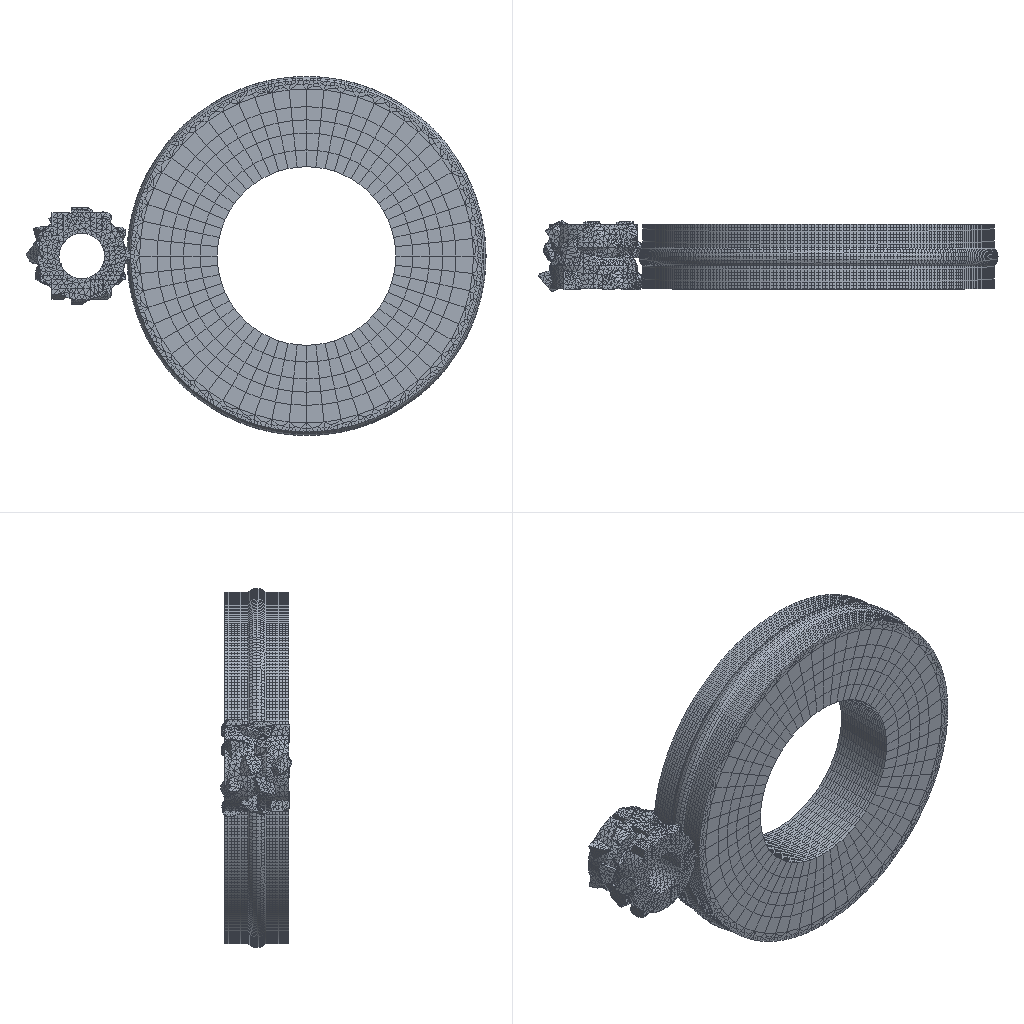Simulation study | abaqus
Set-up summary:
category,name,step,type,value,unit,region
solver,abaqus
solver,version,,,Abaqus/Explicit 2020
units,not stated in the deck,,not stated
analysis,deck,,transient,transient
load_step,Step-1,Step-1,transient,nlgeom=True
contact,interactions,,,general=0 pairs=1 ties=0
load_step,requested,,,1
mesh,nodes,,,26760
mesh,elements,,,38477
element_type,C3D4,,solid,21097
element_type,C3D8R,,solid,17380
load,load commands in deck,,count,3
bc,support commands in deck,,count,12
material,ABQ_JH2_WHITE-CORUNDUM,,in results
material,RIG,,in results
check,setup vs results,,match,"per instance, exact: element labels, types and connectivity; labels of the nodes the elements use; coordinates of those nodes at SINGLE_PRECISION in 2 of 2 instance(s)"
Abaqus input file, long lists of numbers shortened:
*Heading
** Job name: Job-2 Model name: Model-1-Copy
** Generated by: Abaqus/CAE 2020
*Preprint, echo=NO, model=NO, history=NO, contact=NO
**
** PARTS
**
*Part, name=tool
*Node
      1,   1.968,   2.027,  -1.401
      2,   2.361,   1.533,  -1.024
** (4582 more lines like these left out)
*Element, type=C3D4
    1, 2070, 2071, 2072, 2073
    2, 2070, 2074, 2071, 2075
** (21095 more lines like these left out)
*Nset, nset=Set-4, generate
    1,  4584,     1
*Elset, elset=Set-4, generate
     1,  21097,      1
** Section: Section-2
*Solid Section, elset=Set-4, material=rig
,
*End Part
**
*Part, name=work-26
*Node
      1,   12.8,   3.645,         -8.5
      2,   12.8, -0.005,         -8.5
** (22174 more lines like these left out)
*Element, type=C3D8R
  1,    5,  121, 2482,  216,    1,   25, 1931,  120
  2,  121,  122, 2483, 2482,   25,   26, 1932, 1931
** (17378 more lines like these left out)
*Nset, nset=Set-3, generate
     1,  22176,      1
*Elset, elset=Set-3, generate
     1,  17380,      1
** Section: Section-1
*Solid Section, elset=Set-3, material=ABQ_JH2_WHITE-CORUNDUM
,
*End Part
**
**
** ASSEMBLY
**
*Assembly, name=Assembly
**
*Instance, name=work-26-1, part=work-26
       -12.8,       -1.295,           0.
*End Instance
**
*Instance, name=tool-1, part=tool
       -12.8,       -1.295,           0.
*End Instance
**
*Node
      1,  -12.8, 0.02855, -1.5308085e-16
*Node
      2,           0., 2.22044605e-16,           0.
*Nset, nset=Set-4
 1,
*Nset, nset=Set-5
 2,
*Nset, nset=Set-8, instance=work-26-1
   13,   14,   15,   16,  377,  378,  379,  380,  381,  382,  383,  384,  385,  386,  387,  388
  389,  390,  391,  392,  393,  394,  395,  396,  397,  398,  399,  400,  401,  402,  403,  404
** (77 more lines like these left out)
*Elset, elset=Set-8, instance=work-26-1
 1801, 1803, 1805, 1807, 1809, 1811, 1813, 1815, 1817, 1819, 1821, 1823, 1825, 1827, 1829, 1831
 1833, 1835, 1837, 1839, 1841, 1843, 1845, 1847, 1849, 1851, 1853, 1855, 1857, 1859, 1861, 1863
** (73 more lines like these left out)
*Nset, nset=Set-9
 1,
*Nset, nset=b_Set-1, instance=tool-1, generate
    1,  4584,     1
*Elset, elset=b_Set-1, instance=tool-1, generate
     1,  21097,      1
*Nset, nset=m_Set-3
 2,
*Nset, nset=s_Set-6, instance=work-26-1, generate
     1,  22176,      1
*Nset, nset=s_Set-6
 1, 2
*Elset, elset=s_Set-6, instance=work-26-1, generate
     1,  17380,      1
*Nset, nset=s_Set-7, instance=work-26-1, generate
     1,  22176,      1
*Elset, elset=s_Set-7, instance=work-26-1, generate
     1,  17380,      1
*Nset, nset=_PickedSet58, internal
 1,
*Elset, elset=_m_Surf-2_S2, internal, instance=tool-1
    46,    56,   220,   290,   299,   338,   389,   400,   533,   824,   837,   880,   894,   982,  1005,  1118
  1230,  2100,  2297,  2612,  2728,  2745,  2796,  2865,  2967,  3027,  3253,  3258,  3286,  3296,  3448,  3484
** (16 more lines like these left out)
*Elset, elset=_m_Surf-2_S3, internal, instance=tool-1
    81,    85,   101,   115,   174,   180,   309,   458,   515,   553,   667,   770,   814,  1034,  1075,  1085
  1107,  1168,  1176,  1221,  1243,  1263,  1333,  1455,  1460,  1526,  1527,  1542,  1574,  1575,  1587,  1693
** (203 more lines like these left out)
*Elset, elset=_m_Surf-2_S4, internal, instance=tool-1
   146,   299,   431,   477,   545,   587,   645,   955,   960,  1024,  1113,  1260,  1346,  1419,  2008,  2295
  2541,  2645,  2680,  2703,  2796,  2834,  2846,  2860,  2868,  2883,  2890,  2900,  3016,  3025,  3096,  3156
** (18 more lines like these left out)
*Elset, elset=_m_Surf-2_S1, internal, instance=tool-1
    78,   126,   396,   823,   824,   960,  1207,  1833,  2019,  2295,  2497,  2563,  2703,  2715,  2745,  2818
  2857,  2872,  2894,  2903,  2972,  3012,  3029,  3032,  3134,  3205,  3231,  3274,  3294,  3315,  3440,  3452
** (15 more lines like these left out)
*Surface, type=ELEMENT, name=m_Surf-2
_m_Surf-2_S2, S2
_m_Surf-2_S3, S3
_m_Surf-2_S4, S4
_m_Surf-2_S1, S1
*Elset, elset=_s_Surf-1_S6, internal, instance=work-26-1, generate
 1801,  2999,     2
*Elset, elset=_s_Surf-1_S4, internal, instance=work-26-1, generate
 3602,  4800,     2
*Surface, type=ELEMENT, name=s_Surf-1
_s_Surf-1_S6, S6
_s_Surf-1_S4, S4
*Surface, type=NODE, name=s_Set-7_CNS_, internal
s_Set-7, 1.
** Constraint: Constraint-1
*Rigid Body, ref node=_PickedSet58, elset=b_Set-1
*End Assembly
*Amplitude, name=Amp-1, definition=PERIODIC
1,           311.6,              0.,              0.
             0.,         3988.48
*Amplitude, name=Amp-z, definition=PERIODIC
1,           311.6,              0.,              0.
        3988.48,              0.
**
** MATERIALS
**
*Material, name=ABQ_JH2_WHITE-CORUNDUM
*Conductivity
  46., 25.
 32.3,127.
 24.2,227.
 18.9,327.
  13.,527.
*Density
 3.98e-09,
*Depvar, delete=8
      8,
*Specific Heat
 6e+08,
*User Material, constants=32
 3.7e-09, 90160.,   0.93,    0.6,   0.31,    0.6,     0.,     1.
   200., 1.004,    0.2,  2790.,  1460.,     1.,     0.,     0.
  0.005,     1.,  0.005,     0.,    0.2,     0.,     0.,     0.
    13.,     0.,     0.,     0.,     0.,     0.,     0.,     0.
*Material, name=rig
*Conductivity
1000.,
*Density
 3.52e-09,
*Elastic
 1.05e+06, 0.1
*Expansion
 1.26e-06,
*Specific Heat
 4.2e+08,
**
** INTERACTION PROPERTIES
**
*Surface Interaction, name=IntProp-1
*Friction
 0.15,
*Surface Behavior, pressure-overclosure=HARD
** ----------------------------------------------------------------
**
** STEP: Step-1
**
*Step, name=Step-1, nlgeom=YES
*Dynamic, Explicit
, 0.05
*Bulk Viscosity
0.06, 1.2
** Mass Scaling: Semi-Automatic
**               Whole Model
*Fixed Mass Scaling, factor=5000.
**
** BOUNDARY CONDITIONS
**
** Name: BC-1 Type: 速度/角速度
*Boundary, type=VELOCITY
Set-4, 2, 2
Set-4, 4, 4
Set-4, 5, 5, 169.646
Set-4, 6, 6
** Name: BC-2 Type: 速度/角速度
*Boundary, type=VELOCITY
Set-8, 1, 1
Set-8, 2, 2
Set-8, 3, 3
Set-8, 4, 4
Set-8, 5, 5
Set-8, 6, 6
** Name: [REDACTED] : Velocity/Angular velocity
*Boundary, amplitude=Amp-1, type=VELOCITY
Set-9, 1, 1, 1.
** Name: [REDACTED] : Velocity/Angular velocity
*Boundary, amplitude=Amp-z, type=VELOCITY
Set-9, 3, 3, 1.
**
** INTERACTIONS
**
** Interaction: Int-1
*Contact Pair, interaction=IntProp-1, mechanical constraint=KINEMATIC, cpset=Int-1
m_Surf-2, s_Set-7_CNS_
**
** OUTPUT REQUESTS
**
*Restart, write, number interval=1, time marks=NO
**
** FIELD OUTPUT: F-Output-1
**
*Output, field, number interval=50
*Node Output
A, CF, RF, RM, RT, U, V
*Element Output, directions=YES
E, EVF, LE, MISES, MISESMAX, MISESONLY, PE, PEEQ, PEEQMAX, PEEQT, PEEQVAVG, PEMAG, PEQC, PEVAVG, PRESSONLY, S
SEQUT, SF, SFABRIC, SSAVG, STATUS, SVAVG, TEMP, YIELDPOT
*Contact Output
CDISP, CSTRESS
*Output, history, frequency=0
*End Step
Results summary:
result,step,Step-1,completed,increments=67093 time=0.05/0.05
result,analysis,,,transient
result,last_loadstep,,,1
result,analysis steps,,count,1
result,primary field,,,U
result,reaction total,,FX,-1218.07,model units
result,reaction total,,FY,19.269,model units
result,reaction total,,FZ,-3.308,model units